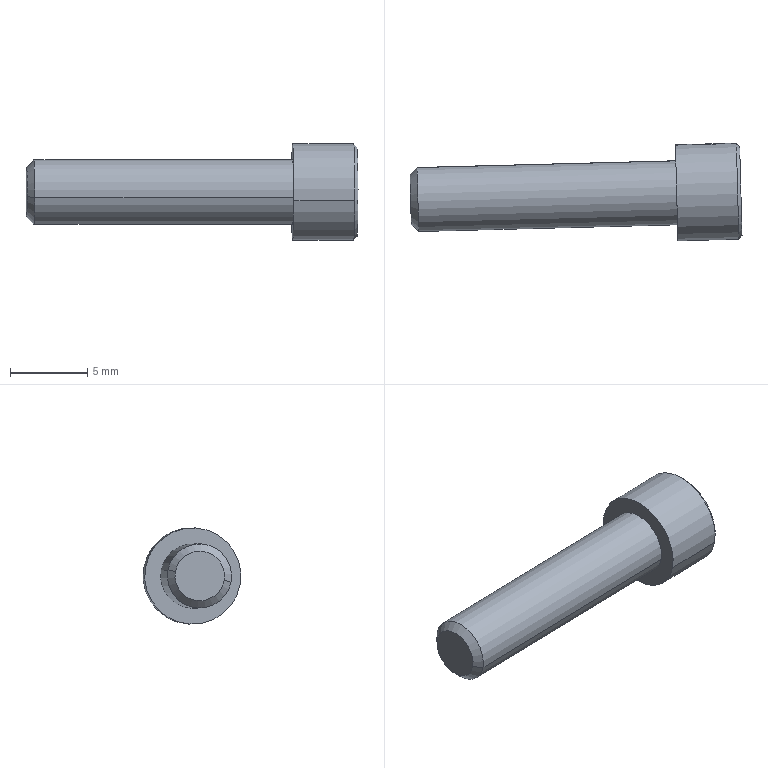Part | STEP file | 1_id1290_x_t | 1 solid | 20 faces | box 21.548 x 6.349 x 6.248 mm | volume 334.04 mm3 | plane 10 | cone 6 | cylinder 4 | commonest cylinder face diameters 4.166 x2 6.248 x2